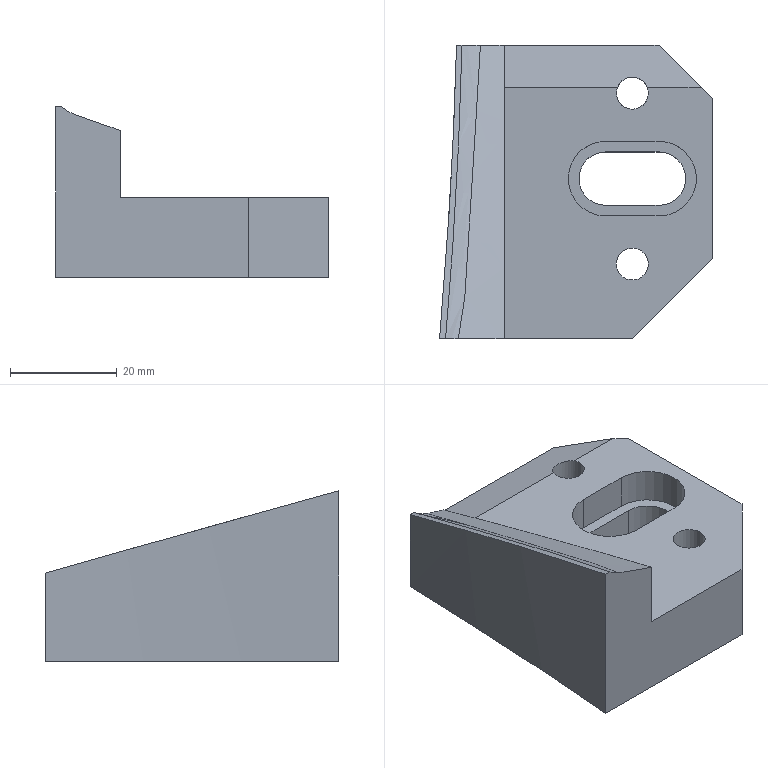Part | NX | features solid 2 | 1 solid | 24 faces | box 51.095 x 55 x 31.918 mm | volume 37917 mm3 | plane 14 | cylinder 6 | spline 4 | commonest cylinder face diameters 6 x2 10 x2 14 x2
STEP:
#1=CARTESIAN_POINT('',(618.,99.,-89.));
#2=VERTEX_POINT('',#1);
#3=CARTESIAN_POINT('',(615.,99.,-89.));
#4=DIRECTION('',(0.,0.,1.));
#5=DIRECTION('',(1.,0.,0.));
#6=AXIS2_PLACEMENT_3D('',#3,#4,#5);
#7=CIRCLE('',#6,3.);
#8=EDGE_CURVE('',#2,#2,#7,.F.);
#9=ORIENTED_EDGE('',*,*,#8,.T.);
#10=EDGE_LOOP('',(#9));
#11=FACE_BOUND('',#10,.T.);
#12=CARTESIAN_POINT('',(620.,122.,-89.));
#13=VERTEX_POINT('',#12);
#14=CARTESIAN_POINT('',(620.,108.,-89.));
#15=VERTEX_POINT('',#14);
#16=CARTESIAN_POINT('',(620.,115.,-89.));
#17=DIRECTION('',(0.,0.,-1.));
#18=DIRECTION('',(0.,-1.,0.));
#19=AXIS2_PLACEMENT_3D('',#16,#17,#18);
#20=CIRCLE('',#19,7.);
#21=EDGE_CURVE('',#13,#15,#20,.T.);
#22=ORIENTED_EDGE('',*,*,#21,.T.);
#23=CARTESIAN_POINT('',(610.,108.,-89.));
#24=VERTEX_POINT('',#23);
#25=CARTESIAN_POINT('',(573.,108.,-89.));
#26=DIRECTION('',(-1.,0.,0.));
#27=VECTOR('',#26,1000.);
#28=LINE('',#25,#27);
#29=EDGE_CURVE('',#15,#24,#28,.T.);
#30=ORIENTED_EDGE('',*,*,#29,.T.);
#31=CARTESIAN_POINT('',(610.,122.,-89.));
#32=VERTEX_POINT('',#31);
#33=CARTESIAN_POINT('',(610.,115.,-89.));
#34=DIRECTION('',(0.,0.,-1.));
#35=DIRECTION('',(0.,-1.,0.));
#36=AXIS2_PLACEMENT_3D('',#33,#34,#35);
#37=CIRCLE('',#36,7.);
#38=EDGE_CURVE('',#32,#24,#37,.F.);
#39=ORIENTED_EDGE('',*,*,#38,.F.);
#40=CARTESIAN_POINT('',(573.,122.,-89.));
#41=DIRECTION('',(-1.,0.,0.));
#42=VECTOR('',#41,1000.);
#43=LINE('',#40,#42);
#44=EDGE_CURVE('',#13,#32,#43,.T.);
#45=ORIENTED_EDGE('',*,*,#44,.F.);
#46=EDGE_LOOP('',(#22,#30,#39,#45));
#47=FACE_BOUND('',#46,.T.);
#48=CARTESIAN_POINT('',(630.,130.,-89.));
#49=VERTEX_POINT('',#48);
#50=CARTESIAN_POINT('',(630.,100.,-89.));
#51=VERTEX_POINT('',#50);
#52=CARTESIAN_POINT('',(630.,90.,-89.));
#53=DIRECTION('',(0.,-1.,0.));
#54=VECTOR('',#53,1000.);
#55=LINE('',#52,#54);
#56=EDGE_CURVE('',#49,#51,#55,.T.);
#57=ORIENTED_EDGE('',*,*,#56,.F.);
#58=CARTESIAN_POINT('',(627.904,132.096,-89.));
#59=VERTEX_POINT('',#58);
#60=CARTESIAN_POINT('',(621.5,138.5,-89.));
#61=DIRECTION('',(-0.7071,0.7071,0.));
#62=VECTOR('',#61,1000.);
#63=LINE('',#60,#62);
#64=EDGE_CURVE('',#49,#59,#63,.T.);
#65=ORIENTED_EDGE('',*,*,#64,.T.);
#66=CARTESIAN_POINT('',(617.793,132.096,-89.));
#67=VERTEX_POINT('',#66);
#68=CARTESIAN_POINT('',(896.,132.096,-89.));
#69=DIRECTION('',(-1.,0.,0.));
#70=VECTOR('',#69,1000.);
#71=LINE('',#68,#70);
#72=EDGE_CURVE('',#59,#67,#71,.T.);
#73=ORIENTED_EDGE('',*,*,#72,.T.);
#74=CARTESIAN_POINT('',(612.207,132.096,-89.));
#75=VERTEX_POINT('',#74);
#76=CARTESIAN_POINT('',(615.,131.,-89.));
#77=DIRECTION('',(0.,0.,1.));
#78=DIRECTION('',(1.,0.,0.));
#79=AXIS2_PLACEMENT_3D('',#76,#77,#78);
#80=CIRCLE('',#79,3.);
#81=EDGE_CURVE('',#67,#75,#80,.F.);
#82=ORIENTED_EDGE('',*,*,#81,.T.);
#83=CARTESIAN_POINT('',(591.,132.096,-89.));
#84=VERTEX_POINT('',#83);
#85=CARTESIAN_POINT('',(896.,132.096,-89.));
#86=DIRECTION('',(-1.,0.,0.));
#87=VECTOR('',#86,1000.);
#88=LINE('',#85,#87);
#89=EDGE_CURVE('',#75,#84,#88,.T.);
#90=ORIENTED_EDGE('',*,*,#89,.T.);
#91=CARTESIAN_POINT('',(591.,85.,-89.));
#92=VERTEX_POINT('',#91);
#93=CARTESIAN_POINT('',(591.,140.,-89.));
#94=DIRECTION('',(0.,1.,0.));
#95=VECTOR('',#94,1000.);
#96=LINE('',#93,#95);
#97=EDGE_CURVE('',#92,#84,#96,.T.);
#98=ORIENTED_EDGE('',*,*,#97,.F.);
#99=CARTESIAN_POINT('',(615.,85.,-89.));
#100=VERTEX_POINT('',#99);
#101=CARTESIAN_POINT('',(573.,85.,-89.));
#102=DIRECTION('',(-1.,0.,0.));
#103=VECTOR('',#102,1000.);
#104=LINE('',#101,#103);
#105=EDGE_CURVE('',#100,#92,#104,.T.);
#106=ORIENTED_EDGE('',*,*,#105,.F.);
#107=CARTESIAN_POINT('',(596.5,66.5,-89.));
#108=DIRECTION('',(-0.7071,-0.7071,0.));
#109=VECTOR('',#108,1000.);
#110=LINE('',#107,#109);
#111=EDGE_CURVE('',#51,#100,#110,.T.);
#112=ORIENTED_EDGE('',*,*,#111,.F.);
#113=EDGE_LOOP('',(#57,#65,#73,#82,#90,#98,#106,#112));
#114=FACE_BOUND('',#113,.T.);
#115=CARTESIAN_POINT('',(573.,90.,-89.));
#116=DIRECTION('',(0.,0.,1.));
#117=DIRECTION('',(0.,-1.,0.));
#118=AXIS2_PLACEMENT_3D('',#115,#116,#117);
#119=PLANE('',#118);
#120=ADVANCED_FACE('',(#11,#47,#114),#119,.T.);
#121=CARTESIAN_POINT('',(610.,120.,-95.5));
#122=VERTEX_POINT('',#121);
#123=CARTESIAN_POINT('',(610.,120.,-104.));
#124=VERTEX_POINT('',#123);
#125=CARTESIAN_POINT('',(610.,120.,-89.));
#126=DIRECTION('',(0.,0.,-1.));
#127=VECTOR('',#126,1000.);
#128=LINE('',#125,#127);
#129=EDGE_CURVE('',#122,#124,#128,.T.);
#130=ORIENTED_EDGE('',*,*,#129,.T.);
#131=CARTESIAN_POINT('',(620.,120.,-104.));
#132=VERTEX_POINT('',#131);
#133=CARTESIAN_POINT('',(610.,120.,-104.));
#134=DIRECTION('',(1.,0.,0.));
#135=VECTOR('',#134,1000.);
#136=LINE('',#133,#135);
#137=EDGE_CURVE('',#124,#132,#136,.T.);
#138=ORIENTED_EDGE('',*,*,#137,.T.);
#139=CARTESIAN_POINT('',(620.,120.,-95.5));
#140=VERTEX_POINT('',#139);
#141=CARTESIAN_POINT('',(620.,120.,-89.));
#142=DIRECTION('',(0.,0.,-1.));
#143=VECTOR('',#142,1000.);
#144=LINE('',#141,#143);
#145=EDGE_CURVE('',#140,#132,#144,.T.);
#146=ORIENTED_EDGE('',*,*,#145,.F.);
#147=CARTESIAN_POINT('',(610.,120.,-95.5));
#148=DIRECTION('',(1.,0.,0.));
#149=VECTOR('',#148,1000.);
#150=LINE('',#147,#149);
#151=EDGE_CURVE('',#122,#140,#150,.T.);
#152=ORIENTED_EDGE('',*,*,#151,.F.);
#153=EDGE_LOOP('',(#130,#138,#146,#152));
#154=FACE_BOUND('',#153,.T.);
#155=CARTESIAN_POINT('',(610.,120.,-89.));
#156=DIRECTION('',(0.,-1.,0.));
#157=DIRECTION('',(-1.,0.,0.));
#158=AXIS2_PLACEMENT_3D('',#155,#156,#157);
#159=PLANE('',#158);
#160=ADVANCED_FACE('',(#154),#159,.T.);
#161=ORIENTED_EDGE('',*,*,#145,.T.);
#162=CARTESIAN_POINT('',(620.,110.,-104.));
#163=VERTEX_POINT('',#162);
#164=CARTESIAN_POINT('',(620.,115.,-104.));
#165=DIRECTION('',(0.,0.,-1.));
#166=DIRECTION('',(0.,-1.,0.));
#167=AXIS2_PLACEMENT_3D('',#164,#165,#166);
#168=CIRCLE('',#167,5.);
#169=EDGE_CURVE('',#132,#163,#168,.T.);
#170=ORIENTED_EDGE('',*,*,#169,.T.);
#171=CARTESIAN_POINT('',(620.,110.,-95.5));
#172=VERTEX_POINT('',#171);
#173=CARTESIAN_POINT('',(620.,110.,-89.));
#174=DIRECTION('',(0.,0.,-1.));
#175=VECTOR('',#174,1000.);
#176=LINE('',#173,#175);
#177=EDGE_CURVE('',#172,#163,#176,.T.);
#178=ORIENTED_EDGE('',*,*,#177,.F.);
#179=CARTESIAN_POINT('',(620.,115.,-95.5));
#180=DIRECTION('',(0.,0.,-1.));
#181=DIRECTION('',(0.,-1.,0.));
#182=AXIS2_PLACEMENT_3D('',#179,#180,#181);
#183=CIRCLE('',#182,5.);
#184=EDGE_CURVE('',#140,#172,#183,.T.);
#185=ORIENTED_EDGE('',*,*,#184,.F.);
#186=EDGE_LOOP('',(#161,#170,#178,#185));
#187=FACE_BOUND('',#186,.T.);
#188=CARTESIAN_POINT('',(620.,115.,-89.));
#189=DIRECTION('',(0.,0.,-1.));
#190=DIRECTION('',(0.,1.,0.));
#191=AXIS2_PLACEMENT_3D('',#188,#189,#190);
#192=CYLINDRICAL_SURFACE('',#191,5.);
#193=ADVANCED_FACE('',(#187),#192,.F.);
#194=CARTESIAN_POINT('',(610.,110.,-95.5));
#195=VERTEX_POINT('',#194);
#196=CARTESIAN_POINT('',(610.,110.,-95.5));
#197=DIRECTION('',(1.,0.,0.));
#198=VECTOR('',#197,1000.);
#199=LINE('',#196,#198);
#200=EDGE_CURVE('',#195,#172,#199,.T.);
#201=ORIENTED_EDGE('',*,*,#200,.T.);
#202=ORIENTED_EDGE('',*,*,#177,.T.);
#203=CARTESIAN_POINT('',(610.,110.,-104.));
#204=VERTEX_POINT('',#203);
#205=CARTESIAN_POINT('',(610.,110.,-104.));
#206=DIRECTION('',(1.,0.,0.));
#207=VECTOR('',#206,1000.);
#208=LINE('',#205,#207);
#209=EDGE_CURVE('',#204,#163,#208,.T.);
#210=ORIENTED_EDGE('',*,*,#209,.F.);
#211=CARTESIAN_POINT('',(610.,110.,-89.));
#212=DIRECTION('',(0.,0.,-1.));
#213=VECTOR('',#212,1000.);
#214=LINE('',#211,#213);
#215=EDGE_CURVE('',#195,#204,#214,.T.);
#216=ORIENTED_EDGE('',*,*,#215,.F.);
#217=EDGE_LOOP('',(#201,#202,#210,#216));
#218=FACE_BOUND('',#217,.T.);
#219=CARTESIAN_POINT('',(610.,110.,-89.));
#220=DIRECTION('',(0.,-1.,0.));
#221=DIRECTION('',(-1.,0.,0.));
#222=AXIS2_PLACEMENT_3D('',#219,#220,#221);
#223=PLANE('',#222);
#224=ADVANCED_FACE('',(#218),#223,.F.);
#225=ORIENTED_EDGE('',*,*,#215,.T.);
#226=CARTESIAN_POINT('',(610.,115.,-104.));
#227=DIRECTION('',(0.,0.,-1.));
#228=DIRECTION('',(0.,-1.,0.));
#229=AXIS2_PLACEMENT_3D('',#226,#227,#228);
#230=CIRCLE('',#229,5.);
#231=EDGE_CURVE('',#204,#124,#230,.T.);
#232=ORIENTED_EDGE('',*,*,#231,.T.);
#233=ORIENTED_EDGE('',*,*,#129,.F.);
#234=CARTESIAN_POINT('',(610.,115.,-95.5));
#235=DIRECTION('',(0.,0.,-1.));
#236=DIRECTION('',(0.,-1.,0.));
#237=AXIS2_PLACEMENT_3D('',#234,#235,#236);
#238=CIRCLE('',#237,5.);
#239=EDGE_CURVE('',#195,#122,#238,.T.);
#240=ORIENTED_EDGE('',*,*,#239,.F.);
#241=EDGE_LOOP('',(#225,#232,#233,#240));
#242=FACE_BOUND('',#241,.T.);
#243=CARTESIAN_POINT('',(610.,115.,-89.));
#244=DIRECTION('',(0.,0.,-1.));
#245=DIRECTION('',(0.,1.,0.));
#246=AXIS2_PLACEMENT_3D('',#243,#244,#245);
#247=CYLINDRICAL_SURFACE('',#246,5.);
#248=ADVANCED_FACE('',(#242),#247,.F.);
#249=CARTESIAN_POINT('',(582.414,85.,-73.515));
#250=VERTEX_POINT('',#249);
#251=CARTESIAN_POINT('',(580.036,85.,-72.082));
#252=VERTEX_POINT('',#251);
#253=CARTESIAN_POINT('',(582.414,85.,-73.515));
#254=CARTESIAN_POINT('',(581.558,85.,-73.162));
#255=CARTESIAN_POINT('',(580.757,85.,-72.679));
#256=CARTESIAN_POINT('',(580.036,85.,-72.082));
#257=B_SPLINE_CURVE_WITH_KNOTS('',3,(#253,#254,#255,#256),.UNSPECIFIED.,.F.,.F.,(4,4),(0.003831,0.0066),.UNSPECIFIED.);
#258=EDGE_CURVE('',#250,#252,#257,.T.);
#259=ORIENTED_EDGE('',*,*,#258,.T.);
#260=CARTESIAN_POINT('',(578.905,85.,-72.082));
#261=VERTEX_POINT('',#260);
#262=CARTESIAN_POINT('',(579.409,85.,-72.082));
#263=DIRECTION('',(-1.,0.,0.));
#264=VECTOR('',#263,1000.);
#265=LINE('',#262,#264);
#266=EDGE_CURVE('',#252,#261,#265,.T.);
#267=ORIENTED_EDGE('',*,*,#266,.T.);
#268=CARTESIAN_POINT('',(578.905,85.,-104.));
#269=VERTEX_POINT('',#268);
#270=CARTESIAN_POINT('',(578.905,85.,-89.));
#271=DIRECTION('',(0.,0.,-1.));
#272=VECTOR('',#271,1000.);
#273=LINE('',#270,#272);
#274=EDGE_CURVE('',#261,#269,#273,.T.);
#275=ORIENTED_EDGE('',*,*,#274,.T.);
#276=CARTESIAN_POINT('',(615.,85.,-104.));
#277=VERTEX_POINT('',#276);
#278=CARTESIAN_POINT('',(573.,85.,-104.));
#279=DIRECTION('',(-1.,0.,0.));
#280=VECTOR('',#279,1000.);
#281=LINE('',#278,#280);
#282=EDGE_CURVE('',#277,#269,#281,.T.);
#283=ORIENTED_EDGE('',*,*,#282,.F.);
#284=CARTESIAN_POINT('',(615.,85.,-89.));
#285=DIRECTION('',(0.,0.,-1.));
#286=VECTOR('',#285,1000.);
#287=LINE('',#284,#286);
#288=EDGE_CURVE('',#100,#277,#287,.T.);
#289=ORIENTED_EDGE('',*,*,#288,.F.);
#290=ORIENTED_EDGE('',*,*,#105,.T.);
#291=CARTESIAN_POINT('',(591.,85.,-76.515));
#292=VERTEX_POINT('',#291);
#293=CARTESIAN_POINT('',(591.,85.,-74.));
#294=DIRECTION('',(0.,0.,-1.));
#295=VECTOR('',#294,1000.);
#296=LINE('',#293,#295);
#297=EDGE_CURVE('',#292,#92,#296,.T.);
#298=ORIENTED_EDGE('',*,*,#297,.F.);
#299=CARTESIAN_POINT('',(591.,85.,-76.515));
#300=CARTESIAN_POINT('',(589.568,85.,-76.019));
#301=CARTESIAN_POINT('',(587.417,85.,-75.28));
#302=CARTESIAN_POINT('',(584.561,85.,-74.264));
#303=CARTESIAN_POINT('',(583.116,85.,-73.805));
#304=CARTESIAN_POINT('',(582.414,85.,-73.515));
#305=B_SPLINE_CURVE_WITH_KNOTS('',3,(#299,#300,#301,#302,#303,#304),.UNSPECIFIED.,.F.,.F.,(4,1,1,4),(0.,0.004547,0.006821,0.009095),.UNSPECIFIED.);
#306=EDGE_CURVE('',#292,#250,#305,.T.);
#307=ORIENTED_EDGE('',*,*,#306,.T.);
#308=EDGE_LOOP('',(#259,#267,#275,#283,#289,#290,#298,#307));
#309=FACE_BOUND('',#308,.T.);
#310=CARTESIAN_POINT('',(621.945,85.,-89.));
#311=DIRECTION('',(0.,1.,0.));
#312=DIRECTION('',(0.,0.,1.));
#313=AXIS2_PLACEMENT_3D('',#310,#311,#312);
#314=PLANE('',#313);
#315=ADVANCED_FACE('',(#309),#314,.F.);
#316=ORIENTED_EDGE('',*,*,#8,.F.);
#317=EDGE_LOOP('',(#316));
#318=FACE_BOUND('',#317,.T.);
#319=CARTESIAN_POINT('',(618.,99.,-104.));
#320=VERTEX_POINT('',#319);
#321=CARTESIAN_POINT('',(615.,99.,-104.));
#322=DIRECTION('',(0.,0.,1.));
#323=DIRECTION('',(1.,0.,0.));
#324=AXIS2_PLACEMENT_3D('',#321,#322,#323);
#325=CIRCLE('',#324,3.);
#326=EDGE_CURVE('',#320,#320,#325,.F.);
#327=ORIENTED_EDGE('',*,*,#326,.T.);
#328=EDGE_LOOP('',(#327));
#329=FACE_BOUND('',#328,.T.);
#330=CARTESIAN_POINT('',(615.,99.,-89.));
#331=DIRECTION('',(0.,0.,-1.));
#332=DIRECTION('',(0.,1.,0.));
#333=AXIS2_PLACEMENT_3D('',#330,#331,#332);
#334=CYLINDRICAL_SURFACE('',#333,3.);
#335=ADVANCED_FACE('',(#318,#329),#334,.F.);
#336=CARTESIAN_POINT('',(582.078,140.,-87.489));
#337=VERTEX_POINT('',#336);
#338=CARTESIAN_POINT('',(582.078,140.,-104.));
#339=VERTEX_POINT('',#338);
#340=CARTESIAN_POINT('',(582.078,140.,-97.234));
#341=DIRECTION('',(0.,0.,-1.));
#342=VECTOR('',#341,1000.);
#343=LINE('',#340,#342);
#344=EDGE_CURVE('',#337,#339,#343,.T.);
#345=ORIENTED_EDGE('',*,*,#344,.F.);
#346=CARTESIAN_POINT('',(583.106,140.,-87.489));
#347=VERTEX_POINT('',#346);
#348=CARTESIAN_POINT('',(582.536,140.,-87.489));
#349=DIRECTION('',(-1.,0.,0.));
#350=VECTOR('',#349,1000.);
#351=LINE('',#348,#350);
#352=EDGE_CURVE('',#337,#347,#351,.F.);
#353=ORIENTED_EDGE('',*,*,#352,.T.);
#354=CARTESIAN_POINT('',(586.549,140.,-89.462));
#355=VERTEX_POINT('',#354);
#356=CARTESIAN_POINT('',(583.106,140.,-87.489));
#357=CARTESIAN_POINT('',(584.098,140.,-88.397));
#358=CARTESIAN_POINT('',(585.278,140.,-89.074));
#359=CARTESIAN_POINT('',(586.549,140.,-89.462));
#360=B_SPLINE_CURVE_WITH_KNOTS('',3,(#356,#357,#358,#359),.UNSPECIFIED.,.F.,.F.,(4,4),(0.006422,0.01041),.UNSPECIFIED.);
#361=EDGE_CURVE('',#347,#355,#360,.T.);
#362=ORIENTED_EDGE('',*,*,#361,.T.);
#363=CARTESIAN_POINT('',(591.,140.,-90.858));
#364=VERTEX_POINT('',#363);
#365=CARTESIAN_POINT('',(586.549,140.,-89.462));
#366=CARTESIAN_POINT('',(588.032,140.,-89.928));
#367=CARTESIAN_POINT('',(589.516,140.,-90.393));
#368=CARTESIAN_POINT('',(591.,140.,-90.858));
#369=B_SPLINE_CURVE_WITH_KNOTS('',3,(#365,#366,#367,#368),.UNSPECIFIED.,.F.,.F.,(4,4),(-0.001537,0.003128),.UNSPECIFIED.);
#370=EDGE_CURVE('',#355,#364,#369,.T.);
#371=ORIENTED_EDGE('',*,*,#370,.T.);
#372=CARTESIAN_POINT('',(591.,140.,-91.123));
#373=VERTEX_POINT('',#372);
#374=CARTESIAN_POINT('',(591.,140.,-74.));
#375=DIRECTION('',(0.,0.,1.));
#376=VECTOR('',#375,1000.);
#377=LINE('',#374,#376);
#378=EDGE_CURVE('',#373,#364,#377,.T.);
#379=ORIENTED_EDGE('',*,*,#378,.F.);
#380=CARTESIAN_POINT('',(620.,140.,-91.123));
#381=VERTEX_POINT('',#380);
#382=CARTESIAN_POINT('',(896.,140.,-91.123));
#383=DIRECTION('',(-1.,0.,0.));
#384=VECTOR('',#383,1000.);
#385=LINE('',#382,#384);
#386=EDGE_CURVE('',#381,#373,#385,.T.);
#387=ORIENTED_EDGE('',*,*,#386,.F.);
#388=CARTESIAN_POINT('',(620.,140.,-104.));
#389=VERTEX_POINT('',#388);
#390=CARTESIAN_POINT('',(620.,140.,-89.));
#391=DIRECTION('',(0.,0.,1.));
#392=VECTOR('',#391,1000.);
#393=LINE('',#390,#392);
#394=EDGE_CURVE('',#389,#381,#393,.T.);
#395=ORIENTED_EDGE('',*,*,#394,.F.);
#396=CARTESIAN_POINT('',(573.,140.,-104.));
#397=DIRECTION('',(1.,0.,0.));
#398=VECTOR('',#397,1000.);
#399=LINE('',#396,#398);
#400=EDGE_CURVE('',#339,#389,#399,.T.);
#401=ORIENTED_EDGE('',*,*,#400,.F.);
#402=EDGE_LOOP('',(#345,#353,#362,#371,#379,#387,#395,#401));
#403=FACE_BOUND('',#402,.T.);
#404=CARTESIAN_POINT('',(573.,140.,-89.));
#405=DIRECTION('',(0.,-1.,0.));
#406=DIRECTION('',(-1.,0.,0.));
#407=AXIS2_PLACEMENT_3D('',#404,#405,#406);
#408=PLANE('',#407);
#409=ADVANCED_FACE('',(#403),#408,.F.);
#410=ORIENTED_EDGE('',*,*,#81,.F.);
#411=CARTESIAN_POINT('',(615.,131.,-88.706));
#412=DIRECTION('',(0.,-0.2594,-0.9658));
#413=DIRECTION('',(0.,0.9658,-0.2594));
#414=AXIS2_PLACEMENT_3D('',#411,#412,#413);
#415=ELLIPSE('',#414,3.106,3.);
#416=EDGE_CURVE('',#75,#67,#415,.T.);
#417=ORIENTED_EDGE('',*,*,#416,.F.);
#418=EDGE_LOOP('',(#410,#417));
#419=FACE_BOUND('',#418,.T.);
#420=CARTESIAN_POINT('',(618.,131.,-104.));
#421=VERTEX_POINT('',#420);
#422=CARTESIAN_POINT('',(615.,131.,-104.));
#423=DIRECTION('',(0.,0.,1.));
#424=DIRECTION('',(1.,0.,0.));
#425=AXIS2_PLACEMENT_3D('',#422,#423,#424);
#426=CIRCLE('',#425,3.);
#427=EDGE_CURVE('',#421,#421,#426,.F.);
#428=ORIENTED_EDGE('',*,*,#427,.T.);
#429=EDGE_LOOP('',(#428));
#430=FACE_BOUND('',#429,.T.);
#431=CARTESIAN_POINT('',(615.,131.,-89.));
#432=DIRECTION('',(0.,0.,-1.));
#433=DIRECTION('',(0.,1.,0.));
#434=AXIS2_PLACEMENT_3D('',#431,#432,#433);
#435=CYLINDRICAL_SURFACE('',#434,3.);
#436=ADVANCED_FACE('',(#419,#430),#435,.F.);
#437=ORIENTED_EDGE('',*,*,#282,.T.);
#438=CARTESIAN_POINT('',(582.078,140.,-104.));
#439=CARTESIAN_POINT('',(581.623,121.633,-104.));
#440=CARTESIAN_POINT('',(580.527,103.287,-104.));
#441=CARTESIAN_POINT('',(578.905,85.,-104.));
#442=B_SPLINE_CURVE_WITH_KNOTS('',3,(#438,#439,#440,#441),.UNSPECIFIED.,.F.,.F.,(4,4),(0.,0.05509),.UNSPECIFIED.);
#443=EDGE_CURVE('',#339,#269,#442,.T.);
#444=ORIENTED_EDGE('',*,*,#443,.F.);
#445=ORIENTED_EDGE('',*,*,#400,.T.);
#446=CARTESIAN_POINT('',(630.,130.,-104.));
#447=VERTEX_POINT('',#446);
#448=CARTESIAN_POINT('',(630.,130.,-104.));
#449=DIRECTION('',(-0.7071,0.7071,0.));
#450=VECTOR('',#449,1000.);
#451=LINE('',#448,#450);
#452=EDGE_CURVE('',#447,#389,#451,.T.);
#453=ORIENTED_EDGE('',*,*,#452,.F.);
#454=CARTESIAN_POINT('',(630.,100.,-104.));
#455=VERTEX_POINT('',#454);
#456=CARTESIAN_POINT('',(630.,90.,-104.));
#457=DIRECTION('',(0.,-1.,0.));
#458=VECTOR('',#457,1000.);
#459=LINE('',#456,#458);
#460=EDGE_CURVE('',#447,#455,#459,.T.);
#461=ORIENTED_EDGE('',*,*,#460,.T.);
#462=CARTESIAN_POINT('',(620.,90.,-104.));
#463=DIRECTION('',(0.7071,0.7071,0.));
#464=VECTOR('',#463,1000.);
#465=LINE('',#462,#464);
#466=EDGE_CURVE('',#277,#455,#465,.T.);
#467=ORIENTED_EDGE('',*,*,#466,.F.);
#468=EDGE_LOOP('',(#437,#444,#445,#453,#461,#467));
#469=FACE_BOUND('',#468,.T.);
#470=ORIENTED_EDGE('',*,*,#427,.F.);
#471=EDGE_LOOP('',(#470));
#472=FACE_BOUND('',#471,.T.);
#473=ORIENTED_EDGE('',*,*,#326,.F.);
#474=EDGE_LOOP('',(#473));
#475=FACE_BOUND('',#474,.T.);
#476=ORIENTED_EDGE('',*,*,#137,.F.);
#477=ORIENTED_EDGE('',*,*,#231,.F.);
#478=ORIENTED_EDGE('',*,*,#209,.T.);
#479=ORIENTED_EDGE('',*,*,#169,.F.);
#480=EDGE_LOOP('',(#476,#477,#478,#479));
#481=FACE_BOUND('',#480,.T.);
#482=CARTESIAN_POINT('',(573.,90.,-104.));
#483=DIRECTION('',(0.,0.,1.));
#484=DIRECTION('',(0.,-1.,0.));
#485=AXIS2_PLACEMENT_3D('',#482,#483,#484);
#486=PLANE('',#485);
#487=ADVANCED_FACE('',(#469,#472,#475,#481),#486,.F.);
#488=CARTESIAN_POINT('',(620.,122.,-95.5));
#489=VERTEX_POINT('',#488);
#490=CARTESIAN_POINT('',(620.,122.,-87.));
#491=DIRECTION('',(0.,0.,-1.));
#492=VECTOR('',#491,1000.);
#493=LINE('',#490,#492);
#494=EDGE_CURVE('',#13,#489,#493,.T.);
#495=ORIENTED_EDGE('',*,*,#494,.F.);
#496=ORIENTED_EDGE('',*,*,#44,.T.);
#497=CARTESIAN_POINT('',(610.,122.,-95.5));
#498=VERTEX_POINT('',#497);
#499=CARTESIAN_POINT('',(610.,122.,-87.));
#500=DIRECTION('',(0.,0.,-1.));
#501=VECTOR('',#500,1000.);
#502=LINE('',#499,#501);
#503=EDGE_CURVE('',#32,#498,#502,.T.);
#504=ORIENTED_EDGE('',*,*,#503,.T.);
#505=CARTESIAN_POINT('',(610.,122.,-95.5));
#506=DIRECTION('',(1.,0.,0.));
#507=VECTOR('',#506,1000.);
#508=LINE('',#505,#507);
#509=EDGE_CURVE('',#498,#489,#508,.T.);
#510=ORIENTED_EDGE('',*,*,#509,.T.);
#511=EDGE_LOOP('',(#495,#496,#504,#510));
#512=FACE_BOUND('',#511,.T.);
#513=CARTESIAN_POINT('',(610.,122.,-87.));
#514=DIRECTION('',(0.,-1.,0.));
#515=DIRECTION('',(0.,0.,-1.));
#516=AXIS2_PLACEMENT_3D('',#513,#514,#515);
#517=PLANE('',#516);
#518=ADVANCED_FACE('',(#512),#517,.T.);
#519=ORIENTED_EDGE('',*,*,#21,.F.);
#520=ORIENTED_EDGE('',*,*,#494,.T.);
#521=CARTESIAN_POINT('',(620.,108.,-95.5));
#522=VERTEX_POINT('',#521);
#523=CARTESIAN_POINT('',(620.,115.,-95.5));
#524=DIRECTION('',(0.,0.,1.));
#525=DIRECTION('',(0.,1.,0.));
#526=AXIS2_PLACEMENT_3D('',#523,#524,#525);
#527=CIRCLE('',#526,7.);
#528=EDGE_CURVE('',#522,#489,#527,.T.);
#529=ORIENTED_EDGE('',*,*,#528,.F.);
#530=CARTESIAN_POINT('',(620.,108.,-87.));
#531=DIRECTION('',(0.,0.,-1.));
#532=VECTOR('',#531,1000.);
#533=LINE('',#530,#532);
#534=EDGE_CURVE('',#15,#522,#533,.T.);
#535=ORIENTED_EDGE('',*,*,#534,.F.);
#536=EDGE_LOOP('',(#519,#520,#529,#535));
#537=FACE_BOUND('',#536,.T.);
#538=CARTESIAN_POINT('',(620.,115.,-87.));
#539=DIRECTION('',(0.,0.,-1.));
#540=DIRECTION('',(0.,1.,0.));
#541=AXIS2_PLACEMENT_3D('',#538,#539,#540);
#542=CYLINDRICAL_SURFACE('',#541,7.);
#543=ADVANCED_FACE('',(#537),#542,.F.);
#544=ORIENTED_EDGE('',*,*,#29,.F.);
#545=ORIENTED_EDGE('',*,*,#534,.T.);
#546=CARTESIAN_POINT('',(610.,108.,-95.5));
#547=VERTEX_POINT('',#546);
#548=CARTESIAN_POINT('',(610.,108.,-95.5));
#549=DIRECTION('',(1.,0.,0.));
#550=VECTOR('',#549,1000.);
#551=LINE('',#548,#550);
#552=EDGE_CURVE('',#547,#522,#551,.T.);
#553=ORIENTED_EDGE('',*,*,#552,.F.);
#554=CARTESIAN_POINT('',(610.,108.,-87.));
#555=DIRECTION('',(0.,0.,-1.));
#556=VECTOR('',#555,1000.);
#557=LINE('',#554,#556);
#558=EDGE_CURVE('',#24,#547,#557,.T.);
#559=ORIENTED_EDGE('',*,*,#558,.F.);
#560=EDGE_LOOP('',(#544,#545,#553,#559));
#561=FACE_BOUND('',#560,.T.);
#562=CARTESIAN_POINT('',(610.,108.,-87.));
#563=DIRECTION('',(0.,-1.,0.));
#564=DIRECTION('',(-1.,0.,0.));
#565=AXIS2_PLACEMENT_3D('',#562,#563,#564);
#566=PLANE('',#565);
#567=ADVANCED_FACE('',(#561),#566,.F.);
#568=ORIENTED_EDGE('',*,*,#503,.F.);
#569=ORIENTED_EDGE('',*,*,#38,.T.);
#570=ORIENTED_EDGE('',*,*,#558,.T.);
#571=CARTESIAN_POINT('',(610.,115.,-95.5));
#572=DIRECTION('',(0.,0.,-1.));
#573=DIRECTION('',(0.,-1.,0.));
#574=AXIS2_PLACEMENT_3D('',#571,#572,#573);
#575=CIRCLE('',#574,7.);
#576=EDGE_CURVE('',#547,#498,#575,.T.);
#577=ORIENTED_EDGE('',*,*,#576,.T.);
#578=EDGE_LOOP('',(#568,#569,#570,#577));
#579=FACE_BOUND('',#578,.T.);
#580=CARTESIAN_POINT('',(610.,115.,-87.));
#581=DIRECTION('',(0.,0.,-1.));
#582=DIRECTION('',(0.,1.,0.));
#583=AXIS2_PLACEMENT_3D('',#580,#581,#582);
#584=CYLINDRICAL_SURFACE('',#583,7.);
#585=ADVANCED_FACE('',(#579),#584,.F.);
#586=ORIENTED_EDGE('',*,*,#239,.T.);
#587=ORIENTED_EDGE('',*,*,#151,.T.);
#588=ORIENTED_EDGE('',*,*,#184,.T.);
#589=ORIENTED_EDGE('',*,*,#200,.F.);
#590=EDGE_LOOP('',(#586,#587,#588,#589));
#591=FACE_BOUND('',#590,.T.);
#592=ORIENTED_EDGE('',*,*,#509,.F.);
#593=ORIENTED_EDGE('',*,*,#576,.F.);
#594=ORIENTED_EDGE('',*,*,#552,.T.);
#595=ORIENTED_EDGE('',*,*,#528,.T.);
#596=EDGE_LOOP('',(#592,#593,#594,#595));
#597=FACE_BOUND('',#596,.T.);
#598=CARTESIAN_POINT('',(620.,115.,-95.5));
#599=DIRECTION('',(0.,0.,1.));
#600=DIRECTION('',(0.,-1.,0.));
#601=AXIS2_PLACEMENT_3D('',#598,#599,#600);
#602=PLANE('',#601);
#603=ADVANCED_FACE('',(#591,#597),#602,.T.);
#604=CARTESIAN_POINT('',(630.,130.,-104.));
#605=DIRECTION('',(0.,0.,-1.));
#606=VECTOR('',#605,1000.);
#607=LINE('',#604,#606);
#608=EDGE_CURVE('',#49,#447,#607,.T.);
#609=ORIENTED_EDGE('',*,*,#608,.F.);
#610=ORIENTED_EDGE('',*,*,#56,.T.);
#611=CARTESIAN_POINT('',(630.,100.,-89.));
#612=DIRECTION('',(0.,0.,1.));
#613=VECTOR('',#612,1000.);
#614=LINE('',#611,#613);
#615=EDGE_CURVE('',#455,#51,#614,.T.);
#616=ORIENTED_EDGE('',*,*,#615,.F.);
#617=ORIENTED_EDGE('',*,*,#460,.F.);
#618=EDGE_LOOP('',(#609,#610,#616,#617));
#619=FACE_BOUND('',#618,.T.);
#620=CARTESIAN_POINT('',(630.,75.,-92.));
#621=DIRECTION('',(1.,0.,0.));
#622=DIRECTION('',(0.,-1.,0.));
#623=AXIS2_PLACEMENT_3D('',#620,#621,#622);
#624=PLANE('',#623);
#625=ADVANCED_FACE('',(#619),#624,.T.);
#626=ORIENTED_EDGE('',*,*,#64,.F.);
#627=ORIENTED_EDGE('',*,*,#608,.T.);
#628=ORIENTED_EDGE('',*,*,#452,.T.);
#629=ORIENTED_EDGE('',*,*,#394,.T.);
#630=CARTESIAN_POINT('',(629.538,130.462,-88.561));
#631=DIRECTION('',(-0.6947,0.6947,-0.1866));
#632=VECTOR('',#631,1000.);
#633=LINE('',#630,#632);
#634=EDGE_CURVE('',#59,#381,#633,.T.);
#635=ORIENTED_EDGE('',*,*,#634,.F.);
#636=EDGE_LOOP('',(#626,#627,#628,#629,#635));
#637=FACE_BOUND('',#636,.T.);
#638=CARTESIAN_POINT('',(630.,130.,-92.));
#639=DIRECTION('',(0.7071,0.7071,0.));
#640=DIRECTION('',(0.7071,-0.7071,0.));
#641=AXIS2_PLACEMENT_3D('',#638,#639,#640);
#642=PLANE('',#641);
#643=ADVANCED_FACE('',(#637),#642,.T.);
#644=ORIENTED_EDGE('',*,*,#111,.T.);
#645=ORIENTED_EDGE('',*,*,#288,.T.);
#646=ORIENTED_EDGE('',*,*,#466,.T.);
#647=ORIENTED_EDGE('',*,*,#615,.T.);
#648=EDGE_LOOP('',(#644,#645,#646,#647));
#649=FACE_BOUND('',#648,.T.);
#650=CARTESIAN_POINT('',(620.,90.,-89.));
#651=DIRECTION('',(0.7071,-0.7071,0.));
#652=DIRECTION('',(-0.7071,-0.7071,0.));
#653=AXIS2_PLACEMENT_3D('',#650,#651,#652);
#654=PLANE('',#653);
#655=ADVANCED_FACE('',(#649),#654,.T.);
#656=ORIENTED_EDGE('',*,*,#274,.F.);
#657=CARTESIAN_POINT('',(578.905,85.,-72.082));
#658=CARTESIAN_POINT('',(580.53,103.319,-77.113));
#659=CARTESIAN_POINT('',(581.623,121.651,-82.308));
#660=CARTESIAN_POINT('',(582.078,140.,-87.489));
#661=B_SPLINE_CURVE_WITH_KNOTS('',3,(#657,#658,#659,#660),.UNSPECIFIED.,.F.,.F.,(4,4),(0.09087,0.148),.UNSPECIFIED.);
#662=EDGE_CURVE('',#261,#337,#661,.T.);
#663=ORIENTED_EDGE('',*,*,#662,.T.);
#664=ORIENTED_EDGE('',*,*,#344,.T.);
#665=ORIENTED_EDGE('',*,*,#443,.T.);
#666=EDGE_LOOP('',(#656,#663,#664,#665));
#667=FACE_BOUND('',#666,.T.);
#668=CARTESIAN_POINT('',(582.078,140.,-87.296));
#669=CARTESIAN_POINT('',(582.078,140.,-119.964));
#670=CARTESIAN_POINT('',(581.623,121.647,-82.013));
#671=CARTESIAN_POINT('',(581.623,121.647,-114.682));
#672=CARTESIAN_POINT('',(580.529,103.308,-76.749));
#673=CARTESIAN_POINT('',(580.529,103.308,-109.418));
#674=CARTESIAN_POINT('',(578.905,85.,-71.525));
#675=CARTESIAN_POINT('',(578.905,85.,-104.194));
#676=B_SPLINE_SURFACE_WITH_KNOTS('',3,1,((#668,#669),(#670,#671),(#672,#673),(#674,#675)),.SURF_OF_LINEAR_EXTRUSION.,.F.,.F.,.F.,(4,4),(2,2),(0.4152,0.4943),(0.,1.),.PIECEWISE_BEZIER_KNOTS.);
#677=ADVANCED_FACE('',(#667),#676,.F.);
#678=ORIENTED_EDGE('',*,*,#378,.T.);
#679=CARTESIAN_POINT('',(591.,140.,-90.858));
#680=CARTESIAN_POINT('',(591.,121.731,-85.834));
#681=CARTESIAN_POINT('',(591.,103.403,-81.017));
#682=CARTESIAN_POINT('',(591.,85.,-76.515));
#683=B_SPLINE_CURVE_WITH_KNOTS('',3,(#679,#680,#681,#682),.UNSPECIFIED.,.F.,.F.,(4,4),(0.,0.05684),.UNSPECIFIED.);
#684=EDGE_CURVE('',#364,#292,#683,.T.);
#685=ORIENTED_EDGE('',*,*,#684,.T.);
#686=ORIENTED_EDGE('',*,*,#297,.T.);
#687=ORIENTED_EDGE('',*,*,#97,.T.);
#688=CARTESIAN_POINT('',(591.,135.71,-89.971));
#689=DIRECTION('',(0.,-0.9658,0.2594));
#690=VECTOR('',#689,1000.);
#691=LINE('',#688,#690);
#692=EDGE_CURVE('',#373,#84,#691,.T.);
#693=ORIENTED_EDGE('',*,*,#692,.F.);
#694=EDGE_LOOP('',(#678,#685,#686,#687,#693));
#695=FACE_BOUND('',#694,.T.);
#696=CARTESIAN_POINT('',(591.,140.,-74.));
#697=DIRECTION('',(-1.,0.,0.));
#698=DIRECTION('',(0.,0.,1.));
#699=AXIS2_PLACEMENT_3D('',#696,#697,#698);
#700=PLANE('',#699);
#701=ADVANCED_FACE('',(#695),#700,.F.);
#702=ORIENTED_EDGE('',*,*,#72,.F.);
#703=ORIENTED_EDGE('',*,*,#634,.T.);
#704=ORIENTED_EDGE('',*,*,#386,.T.);
#705=ORIENTED_EDGE('',*,*,#692,.T.);
#706=ORIENTED_EDGE('',*,*,#89,.F.);
#707=ORIENTED_EDGE('',*,*,#416,.T.);
#708=EDGE_LOOP('',(#702,#703,#704,#705,#706,#707));
#709=FACE_BOUND('',#708,.T.);
#710=CARTESIAN_POINT('',(896.,140.337,-91.214));
#711=DIRECTION('',(0.,-0.2594,-0.9658));
#712=DIRECTION('',(0.,0.9658,-0.2594));
#713=AXIS2_PLACEMENT_3D('',#710,#711,#712);
#714=PLANE('',#713);
#715=ADVANCED_FACE('',(#709),#714,.F.);
#716=ORIENTED_EDGE('',*,*,#361,.F.);
#717=CARTESIAN_POINT('',(583.106,140.,-87.489));
#718=CARTESIAN_POINT('',(582.68,121.651,-82.308));
#719=CARTESIAN_POINT('',(581.606,103.328,-77.116));
#720=CARTESIAN_POINT('',(580.036,85.,-72.082));
#721=B_SPLINE_CURVE_WITH_KNOTS('',3,(#717,#718,#719,#720),.UNSPECIFIED.,.F.,.F.,(4,4),(0.,0.05721),.UNSPECIFIED.);
#722=EDGE_CURVE('',#347,#252,#721,.T.);
#723=ORIENTED_EDGE('',*,*,#722,.T.);
#724=ORIENTED_EDGE('',*,*,#258,.F.);
#725=CARTESIAN_POINT('',(583.621,92.758,-75.903));
#726=VERTEX_POINT('',#725);
#727=CARTESIAN_POINT('',(582.414,85.,-73.515));
#728=CARTESIAN_POINT('',(582.74,87.466,-74.25));
#729=CARTESIAN_POINT('',(583.141,90.05,-75.05));
#730=CARTESIAN_POINT('',(583.621,92.758,-75.903));
#731=B_SPLINE_CURVE_WITH_KNOTS('',3,(#727,#728,#729,#730),.UNSPECIFIED.,.F.,.F.,(4,4),(0.02883,1.),.UNSPECIFIED.);
#732=EDGE_CURVE('',#250,#726,#731,.T.);
#733=ORIENTED_EDGE('',*,*,#732,.T.);
#734=CARTESIAN_POINT('',(583.621,92.758,-75.903));
#735=CARTESIAN_POINT('',(583.872,96.612,-76.969));
#736=CARTESIAN_POINT('',(584.252,102.467,-78.604));
#737=CARTESIAN_POINT('',(584.751,110.369,-80.842));
#738=CARTESIAN_POINT('',(585.129,116.456,-82.583));
#739=CARTESIAN_POINT('',(585.484,122.255,-84.257));
#740=CARTESIAN_POINT('',(585.96,130.125,-86.547));
#741=CARTESIAN_POINT('',(586.313,136.037,-88.289));
#742=CARTESIAN_POINT('',(586.549,140.,-89.462));
#743=B_SPLINE_CURVE_WITH_KNOTS('',3,(#734,#735,#736,#737,#738,#739,#740,#741,#742),.UNSPECIFIED.,.F.,.F.,(4,1,1,1,1,1,4),(0.,0.25,0.375,0.5,0.625,0.75,1.),.UNSPECIFIED.);
#744=EDGE_CURVE('',#726,#355,#743,.T.);
#745=ORIENTED_EDGE('',*,*,#744,.T.);
#746=EDGE_LOOP('',(#716,#723,#724,#733,#745));
#747=FACE_BOUND('',#746,.T.);
#748=CARTESIAN_POINT('',(586.582,140.334,-89.565));
#749=CARTESIAN_POINT('',(586.265,140.37,-89.468));
#750=CARTESIAN_POINT('',(585.632,140.442,-89.274));
#751=CARTESIAN_POINT('',(584.734,140.585,-88.855));
#752=CARTESIAN_POINT('',(583.883,140.75,-88.356));
#753=CARTESIAN_POINT('',(583.372,140.88,-87.949));
#754=CARTESIAN_POINT('',(583.116,140.945,-87.745));
#755=CARTESIAN_POINT('',(586.412,135.615,-88.209));
#756=CARTESIAN_POINT('',(586.096,135.653,-88.112));
#757=CARTESIAN_POINT('',(585.465,135.729,-87.917));
#758=CARTESIAN_POINT('',(584.571,135.877,-87.499));
#759=CARTESIAN_POINT('',(583.723,136.046,-87.));
#760=CARTESIAN_POINT('',(583.214,136.178,-86.594));
#761=CARTESIAN_POINT('',(582.96,136.244,-86.392));
#762=CARTESIAN_POINT('',(586.07,126.179,-85.496));
#763=CARTESIAN_POINT('',(585.758,126.22,-85.398));
#764=CARTESIAN_POINT('',(585.132,126.302,-85.204));
#765=CARTESIAN_POINT('',(584.245,126.46,-84.786));
#766=CARTESIAN_POINT('',(583.404,126.638,-84.29));
#767=CARTESIAN_POINT('',(582.9,126.775,-83.886));
#768=CARTESIAN_POINT('',(582.647,126.843,-83.684));
#769=CARTESIAN_POINT('',(585.25,112.074,-81.453));
#770=CARTESIAN_POINT('',(584.941,112.121,-81.355));
#771=CARTESIAN_POINT('',(584.323,112.213,-81.16));
#772=CARTESIAN_POINT('',(583.448,112.385,-80.744));
#773=CARTESIAN_POINT('',(582.619,112.575,-80.25));
#774=CARTESIAN_POINT('',(582.121,112.719,-79.849));
#775=CARTESIAN_POINT('',(581.873,112.791,-79.649));
#776=CARTESIAN_POINT('',(584.216,98.004,-77.426));
#777=CARTESIAN_POINT('',(583.911,98.056,-77.328));
#778=CARTESIAN_POINT('',(583.301,98.159,-77.132));
#779=CARTESIAN_POINT('',(582.438,98.345,-76.717));
#780=CARTESIAN_POINT('',(581.621,98.548,-76.227));
#781=CARTESIAN_POINT('',(581.13,98.699,-75.829));
#782=CARTESIAN_POINT('',(580.885,98.775,-75.631));
#783=CARTESIAN_POINT('',(583.32,88.66,-74.766));
#784=CARTESIAN_POINT('',(583.017,88.714,-74.668));
#785=CARTESIAN_POINT('',(582.412,88.824,-74.471));
#786=CARTESIAN_POINT('',(581.557,89.018,-74.057));
#787=CARTESIAN_POINT('',(580.747,89.229,-73.568));
#788=CARTESIAN_POINT('',(580.261,89.384,-73.172));
#789=CARTESIAN_POINT('',(580.018,89.462,-72.974));
#790=CARTESIAN_POINT('',(582.871,83.987,-73.436));
#791=CARTESIAN_POINT('',(582.57,84.044,-73.338));
#792=CARTESIAN_POINT('',(581.967,84.157,-73.141));
#793=CARTESIAN_POINT('',(581.116,84.354,-72.727));
#794=CARTESIAN_POINT('',(580.31,84.569,-72.238));
#795=CARTESIAN_POINT('',(579.826,84.726,-71.844));
#796=CARTESIAN_POINT('',(579.585,84.805,-71.646));
#797=B_SPLINE_SURFACE_WITH_KNOTS('',3,3,((#748,#749,#750,#751,#752,#753,#754),(#755,#756,#757,#758,#759,#760,#761),(#762,#763,#764,#765,#766,#767,#768),(#769,#770,#771,#772,#773,#774,#775),(#776,#777,#778,#779,#780,#781,#782),(#783,#784,#785,#786,#787,#788,#789),(#790,#791,#792,#793,#794,#795,#796)),.UNSPECIFIED.,.F.,.F.,.F.,(4,1,1,1,4),(4,1,1,1,4),(0.2884,0.3033,0.3182,0.3332,0.3481),(-0.02104,0.1403,0.3016,0.463,0.6243),.UNSPECIFIED.);
#798=ADVANCED_FACE('',(#747),#797,.F.);
#799=ORIENTED_EDGE('',*,*,#306,.F.);
#800=ORIENTED_EDGE('',*,*,#684,.F.);
#801=ORIENTED_EDGE('',*,*,#370,.F.);
#802=ORIENTED_EDGE('',*,*,#744,.F.);
#803=ORIENTED_EDGE('',*,*,#732,.F.);
#804=EDGE_LOOP('',(#799,#800,#801,#802,#803));
#805=FACE_BOUND('',#804,.T.);
#806=CARTESIAN_POINT('',(594.921,139.922,-92.065));
#807=CARTESIAN_POINT('',(593.443,140.078,-91.647));
#808=CARTESIAN_POINT('',(591.321,140.305,-91.039));
#809=CARTESIAN_POINT('',(588.812,140.569,-90.335));
#810=CARTESIAN_POINT('',(587.296,140.734,-89.894));
#811=CARTESIAN_POINT('',(586.472,140.817,-89.674));
#812=CARTESIAN_POINT('',(585.959,140.88,-89.501));
#813=CARTESIAN_POINT('',(594.214,120.886,-86.656));
#814=CARTESIAN_POINT('',(592.759,121.075,-86.236));
#815=CARTESIAN_POINT('',(590.669,121.349,-85.623));
#816=CARTESIAN_POINT('',(588.198,121.669,-84.915));
#817=CARTESIAN_POINT('',(586.705,121.867,-84.471));
#818=CARTESIAN_POINT('',(585.894,121.968,-84.25));
#819=CARTESIAN_POINT('',(585.388,122.042,-84.076));
#820=CARTESIAN_POINT('',(592.858,101.941,-81.288));
#821=CARTESIAN_POINT('',(591.428,102.165,-80.866));
#822=CARTESIAN_POINT('',(589.374,102.489,-80.252));
#823=CARTESIAN_POINT('',(586.945,102.867,-79.54));
#824=CARTESIAN_POINT('',(585.477,103.1,-79.095));
#825=CARTESIAN_POINT('',(584.679,103.221,-78.873));
#826=CARTESIAN_POINT('',(584.182,103.306,-78.699));
#827=CARTESIAN_POINT('',(590.857,83.145,-76.013));
#828=CARTESIAN_POINT('',(589.45,83.396,-75.587));
#829=CARTESIAN_POINT('',(587.43,83.76,-74.967));
#830=CARTESIAN_POINT('',(585.041,84.186,-74.248));
#831=CARTESIAN_POINT('',(583.597,84.448,-73.799));
#832=CARTESIAN_POINT('',(582.813,84.585,-73.574));
#833=CARTESIAN_POINT('',(582.324,84.68,-73.4));
#834=B_SPLINE_SURFACE_WITH_KNOTS('',3,3,((#806,#807,#808,#809,#810,#811,#812),(#813,#814,#815,#816,#817,#818,#819),(#820,#821,#822,#823,#824,#825,#826),(#827,#828,#829,#830,#831,#832,#833)),.UNSPECIFIED.,.F.,.F.,.F.,(4,4),(4,1,1,1,4),(0.5033,0.5265),(0.1141,0.2694,0.3341,0.3794,0.4247),.UNSPECIFIED.);
#835=ADVANCED_FACE('',(#805),#834,.F.);
#836=ORIENTED_EDGE('',*,*,#266,.F.);
#837=ORIENTED_EDGE('',*,*,#722,.F.);
#838=ORIENTED_EDGE('',*,*,#352,.F.);
#839=ORIENTED_EDGE('',*,*,#662,.F.);
#840=EDGE_LOOP('',(#836,#837,#838,#839));
#841=FACE_BOUND('',#840,.T.);
#842=CARTESIAN_POINT('',(583.212,140.,-87.489));
#843=CARTESIAN_POINT('',(582.068,140.,-87.489));
#844=CARTESIAN_POINT('',(582.759,121.648,-82.307));
#845=CARTESIAN_POINT('',(581.614,121.648,-82.307));
#846=CARTESIAN_POINT('',(581.668,103.325,-77.115));
#847=CARTESIAN_POINT('',(580.523,103.325,-77.115));
#848=CARTESIAN_POINT('',(580.043,85.,-72.082));
#849=CARTESIAN_POINT('',(578.898,85.,-72.082));
#850=B_SPLINE_SURFACE_WITH_KNOTS('',3,1,((#842,#843),(#844,#845),(#846,#847),(#848,#849)),.SURF_OF_LINEAR_EXTRUSION.,.F.,.F.,.F.,(4,4),(2,2),(-0.0009872,0.999),(0.,1.),.PIECEWISE_BEZIER_KNOTS.);
#851=ADVANCED_FACE('',(#841),#850,.F.);
#852=CLOSED_SHELL('',(#120,#160,#193,#224,#248,#315,#335,#409,#436,#487,#518,#543,#567,#585,#603,#625,#643,#655,#677,#701,#715,#798,#835,#851));
#853=MANIFOLD_SOLID_BREP('',#852);
#854=(LENGTH_UNIT()NAMED_UNIT(*)SI_UNIT(.MILLI.,.METRE.));
#855=UNCERTAINTY_MEASURE_WITH_UNIT(LENGTH_MEASURE(0.0508),#854,'','');
#856=(NAMED_UNIT(*)PLANE_ANGLE_UNIT()SI_UNIT($,.RADIAN.));
#857=(NAMED_UNIT(*)SI_UNIT($,.STERADIAN.)SOLID_ANGLE_UNIT());
#858=(GEOMETRIC_REPRESENTATION_CONTEXT(3)GLOBAL_UNCERTAINTY_ASSIGNED_CONTEXT((#855))GLOBAL_UNIT_ASSIGNED_CONTEXT((#854,#856,#857))REPRESENTATION_CONTEXT('',''));
#859=ADVANCED_BREP_SHAPE_REPRESENTATION('',(#853),#858);